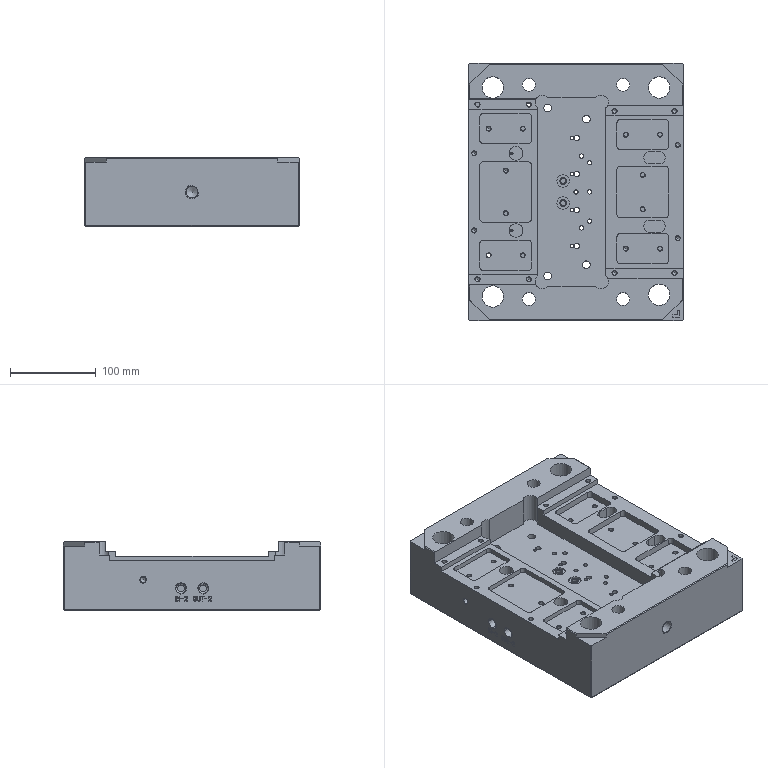NC program | PowerMill | posted with a generic post | part box 250 x 300 x 80 mm
Lines 1 to 768 of 17319:
%
O0001
N104 ( POWERMILL CB  : 2026004.0)
N105 ( POST VER      : 2026.0.0.5161)
N106 ( OPTION FILE   : FANUC)
N107 ( OUTPUT WORKPLANE : 1)
N108 (  )
N109 ( TOOL LIST )
N110 (----------------------------------)
N111 ( NO. | ID   | DIA.| TIP RAD|LENGTH)
N112 (----------------------------------)
N113 (    1|D8_1_1| 8.0 |  0.0   |100.24)
N114 (----------------------------------)
N115 (  )
N116 ( NUMBER OF TOOLPATHS: 1.0 )
N117 ( ESTIMATED PROGRAM DURATION: 0 HOURS 1 MIN 10 SEC)
N118 (  )
N119 G00 G21 G80 G40 G17
N120 G90
N121 G54
N122 G53 Z0.0
N123 (---------------)
N124 ( START TOOLPATH : 07中光-D8-等高 )
N125 (---------------)
N126 ( TOOL NO.    :1 )
N127 ( TOOL TYPE   : ENDMILL)
N128 ( TOOL ID     : D8_1_1)
N129 ( TOOL DIA    : 8.0 LENGTH 100.24)
N130 T1
N131 M6
N132 S3500 M03
N133 G00 G90 X82.0118 Y-12.1812
N134 G43 Z22.0 H1
N135
N136 G05 P10000 R8
N137 Z0.151
N138 G01 X82.0182 Y-12.2863 Z0.1455 F2100.0
N139 X82.0436 Y-12.4854 Z0.1349
N140 X82.0833 Y-12.687 Z0.1242
N141 X82.1478 Y-12.9174 Z0.1116
N142 X82.2928 Y-13.2849 Z0.0909
N143 X82.3993 Y-13.4891 Z0.0788
N144 X82.5476 Y-13.7209 Z0.0644
N145 X82.6911 Y-13.9087 Z0.052
N146 X82.9473 Y-14.183 Z0.0324
N147 X83.1294 Y-14.3414 Z0.0197
N148 X83.3239 Y-14.4841 Z0.0071
N149 X83.5429 Y-14.6176 Z-0.0064
N150 X83.7468 Y-14.721 Z-0.0183
N151 X83.9442 Y-14.8037 Z-0.0296
N152 X84.1906 Y-14.8839 Z-0.0431
N153 X84.5463 Y-14.9624 Z-0.0622
N154 X84.7454 Y-14.9854 Z-0.0727
N155 X84.946 Y-14.9952 Z-0.0833
N156 X85.1462 Y-14.9917 Z-0.0938
N157 X85.3458 Y-14.9751 Z-0.1042
N158 X85.5469 Y-14.9448 Z-0.1149
N159 X85.8094 Y-14.8839 Z-0.129
N160 X86.1453 Y-14.7681 F3500.0
N161 X86.3491 Y-14.6747
N162 X86.545 Y-14.5665
N163 X86.6761 Y-14.4841
N164 X86.9448 Y-14.2779
N165 X87.1514 Y-14.0844
N166 X87.3445 Y-13.8667
N167 X87.4785 Y-13.6846
N168 X87.6007 Y-13.4891
N169 X87.7443 Y-13.1999
N170 X87.8634 Y-12.8851
N171 X87.9167 Y-12.6871
N172 X87.9565 Y-12.4854
N173 X87.9818 Y-12.2863
N174 X87.994 Y-12.0857
N175 X87.9929 Y-11.8855
N176 X87.9787 Y-11.6859
N177 X87.9508 Y-11.4848
N178 X87.9095 Y-11.2862
N179 X87.8526 Y-11.0839
N180 X87.7443 Y-10.8001
N181 X87.5864 Y-10.4867
N182 X87.4717 Y-10.3056
N183 X87.3052 Y-10.0869
N184 X87.1326 Y-9.8969
N185 X86.9042 Y-9.6872
N186 X86.7294 Y-9.5539
N187 X86.545 Y-9.4335
N188 X86.2725 Y-9.2874
N189 X85.9478 Y-9.1585
N190 X85.7455 Y-9.099
N191 X85.5469 Y-9.0552
N192 X85.3458 Y-9.0249
N193 X85.1462 Y-9.0083
N194 X84.946 Y-9.0048
N195 X84.7454 Y-9.0146
N196 X84.5463 Y-9.0376
N197 X84.1466 Y-9.1279
N198 X83.9442 Y-9.1963
N199 X83.7274 Y-9.2874
N200 X83.5335 Y-9.3874
N201 X83.3471 Y-9.5013
N202 X83.0958 Y-9.6872
N203 X82.9473 Y-9.817
N204 X82.6949 Y-10.0869
N205 X82.5476 Y-10.2791
N206 X82.4136 Y-10.4867
N207 X82.3085 Y-10.6827
N208 X82.2181 Y-10.8864
N209 X82.1478 Y-11.0827
N210 X82.0905 Y-11.2862
N211 X82.0492 Y-11.4848
N212 X82.0213 Y-11.6859
N213 X82.0071 Y-11.8855
N214 X82.006 Y-12.0857
N215 X82.0182 Y-12.2863
N216 X82.0436 Y-12.4854
N217 X82.0833 Y-12.687
N218 X82.1478 Y-12.9174
N219 X82.2928 Y-13.2849
N220 X82.3993 Y-13.4891
N221 X82.5476 Y-13.7209
N222 X82.6911 Y-13.9087
N223 X82.9473 Y-14.183
N224 X83.1294 Y-14.3414
N225 X83.3239 Y-14.4841
N226 X83.5429 Y-14.6176
N227 X83.7468 Y-14.721
N228 X83.9442 Y-14.8037
N229 X84.1906 Y-14.8839
N230 X84.5463 Y-14.9624
N231 X84.7454 Y-14.9854
N232 X84.946 Y-14.9952
N233 X85.1462 Y-14.9917
N234 X85.3458 Y-14.9751
N235 X85.5469 Y-14.9448
N236 X85.8094 Y-14.8839
N237 X85.979 Y-14.8306 Z-0.1307
N238 X86.1485 Y-14.7667 Z-0.1324
N239 X86.3491 Y-14.6747 Z-0.1345
N240 X86.5471 Y-14.5652 Z-0.1366
N241 X86.6761 Y-14.4841 Z-0.1381
N242 X86.9481 Y-14.275 Z-0.1413
N243 X87.1513 Y-14.0844 Z-0.1439
N244 X87.3467 Y-13.8639 Z-0.1467
N245 X87.4785 Y-13.6846 Z-0.1488
N246 X87.6007 Y-13.4891 Z-0.151
N247 X87.7464 Y-13.1951 Z-0.1541
N248 X87.8634 Y-12.8851 Z-0.1572
N249 X87.9167 Y-12.6871 Z-0.1591
N250 X87.9564 Y-12.4854 Z-0.1611
N251 X87.9818 Y-12.2863 Z-0.163
N252 X87.994 Y-12.0857 Z-0.1649
N253 X87.9929 Y-11.8855 Z-0.1667
N254 X87.9787 Y-11.6859 Z-0.1686
N255 X87.9508 Y-11.4848 Z-0.1705
N256 X87.9095 Y-11.2862 Z-0.1725
N257 X87.8526 Y-11.0839 Z-0.1744
N258 X87.7819 Y-10.8864 Z-0.1764
N259 X87.6695 Y-10.6412 Z-0.179
N260 X87.5864 Y-10.4867 Z-0.1806
N261 X87.4717 Y-10.3056 Z-0.1826
N262 X87.3445 Y-10.1333 Z-0.1846
N263 X87.1326 Y-9.8969 Z-0.1876
N264 X86.9042 Y-9.6872 Z-0.1906
N265 X86.7294 Y-9.5539 Z-0.1926
N266 X86.545 Y-9.4335 Z-0.1947
N267 X86.2725 Y-9.2874 Z-0.1976
N268 X85.9478 Y-9.1585 Z-0.2009
N269 X85.7455 Y-9.099 Z-0.2029
N270 X85.5469 Y-9.0552 Z-0.2048
N271 X85.3458 Y-9.0249 Z-0.2067
N272 X85.1462 Y-9.0083 Z-0.2086
N273 X84.9429 Y-9.0049 Z-0.2106
N274 X84.7454 Y-9.0146 Z-0.2124
N275 X84.5463 Y-9.0376 Z-0.2143
N276 X84.3432 Y-9.076 Z-0.2163
N277 X84.1433 Y-9.1288 Z-0.2182
N278 X83.9442 Y-9.1963 Z-0.2202
N279 X83.7274 Y-9.2874 Z-0.2224
N280 X83.5305 Y-9.389 Z-0.2245
N281 X83.345 Y-9.5026 Z-0.2265
N282 X83.0958 Y-9.6872 Z-0.2295
N283 X82.9432 Y-9.8211 Z-0.2314
N284 X82.8145 Y-9.9498 Z-0.2331
N285 X82.6949 Y-10.0869 Z-0.2348
N286 X82.5453 Y-10.2822 Z-0.2371
N287 X82.4136 Y-10.4867 Z-0.2394
N288 X82.3085 Y-10.6827 Z-0.2415
N289 X82.2181 Y-10.8864 Z-0.2436
N290 X82.1467 Y-11.0858 Z-0.2456
N291 X82.0905 Y-11.2862 Z-0.2476
N292 X82.0492 Y-11.4848 Z-0.2495
N293 X82.0213 Y-11.6859 Z-0.2514
N294 X82.0071 Y-11.8855 Z-0.2533
N295 X82.006 Y-12.0857 Z-0.2552
N296 X82.0182 Y-12.2863 Z-0.2571
N297 X82.0436 Y-12.4854 Z-0.259
N298 X82.0833 Y-12.687 Z-0.2609
N299 X82.1366 Y-12.8851 Z-0.2628
N300 X82.2075 Y-13.0878 Z-0.2649
N301 X82.2928 Y-13.2849 Z-0.2669
N302 X82.3993 Y-13.4891 Z-0.2691
N303 X82.5215 Y-13.6846 Z-0.2712
N304 X82.6911 Y-13.9087 Z-0.2739
N305 X82.9473 Y-14.183 Z-0.2774
N306 X83.1294 Y-14.3414 Z-0.2797
N307 X83.3239 Y-14.4841 Z-0.282
N308 X83.546 Y-14.6192 Z-0.2844
N309 X83.7499 Y-14.7223 Z-0.2866
N310 X83.9442 Y-14.8037 Z-0.2886
N311 X84.1466 Y-14.8721 Z-0.2906
N312 X84.3449 Y-14.9243 Z-0.2925
N313 X84.5463 Y-14.9624 Z-0.2944
N314 X84.7454 Y-14.9854 Z-0.2963
N315 X84.946 Y-14.9952 Z-0.2982
N316 X85.1462 Y-14.9917 Z-0.3001
N317 X85.3458 Y-14.9751 Z-0.302
N318 X85.5469 Y-14.9448 Z-0.3039
N319 X85.8094 Y-14.8839 Z-0.3065
N320 X85.979 Y-14.8306 Z-0.3081
N321 X86.1485 Y-14.7667 Z-0.3098
N322 X86.3521 Y-14.6731 Z-0.3119
N323 X86.5471 Y-14.5652 Z-0.314
N324 X86.6761 Y-14.4841 Z-0.3155
N325 X86.9481 Y-14.275 Z-0.3187
N326 X87.1513 Y-14.0844 Z-0.3213
N327 X87.3467 Y-13.8639 Z-0.3241
N328 X87.4785 Y-13.6846 Z-0.3262
N329 X87.6007 Y-13.4891 Z-0.3284
N330 X87.7464 Y-13.1951 Z-0.3315
N331 X87.8634 Y-12.8851 Z-0.3346
N332 X87.9167 Y-12.6871 Z-0.3365
N333 X87.9564 Y-12.4854 Z-0.3385
N334 X87.9818 Y-12.2863 Z-0.3404
N335 X87.994 Y-12.0857 Z-0.3423
N336 X87.9929 Y-11.8855 Z-0.3442
N337 X87.9787 Y-11.6859 Z-0.346
N338 X87.9508 Y-11.4848 Z-0.348
N339 X87.9095 Y-11.2862 Z-0.3499
N340 X87.8526 Y-11.0839 Z-0.3519
N341 X87.7819 Y-10.8864 Z-0.3538
N342 X87.6695 Y-10.6412 Z-0.3564
N343 X87.5864 Y-10.4867 Z-0.358
N344 X87.4717 Y-10.3056 Z-0.36
N345 X87.3445 Y-10.1333 Z-0.3621
N346 X87.1326 Y-9.8969 Z-0.3651
N347 X86.9042 Y-9.6872 Z-0.368
N348 X86.7294 Y-9.5539 Z-0.3701
N349 X86.545 Y-9.4335 Z-0.3721
N350 X86.2725 Y-9.2874 Z-0.375
N351 X85.9478 Y-9.1585 Z-0.3783
N352 X85.7455 Y-9.099 Z-0.3803
N353 X85.5469 Y-9.0552 Z-0.3822
N354 X85.3458 Y-9.0249 Z-0.3842
N355 X85.1462 Y-9.0083 Z-0.3861
N356 X84.9429 Y-9.0049 Z-0.388
N357 X84.7454 Y-9.0146 Z-0.3898
N358 X84.54 Y-9.0388 Z-0.3918
N359 X84.3401 Y-9.0766 Z-0.3937
N360 X84.1433 Y-9.1288 Z-0.3956
N361 X83.9442 Y-9.1963 Z-0.3976
N362 X83.7274 Y-9.2874 Z-0.3998
N363 X83.5335 Y-9.3874 Z-0.4019
N364 X83.345 Y-9.5026 Z-0.404
N365 X83.0958 Y-9.6872 Z-0.4069
N366 X82.9432 Y-9.8211 Z-0.4088
N367 X82.8145 Y-9.9498 Z-0.4105
N368 X82.6949 Y-10.0869 Z-0.4122
N369 X82.5453 Y-10.2822 Z-0.4145
N370 X82.4136 Y-10.4867 Z-0.4168
N371 X82.3085 Y-10.6827 Z-0.4189
N372 X82.2181 Y-10.8864 Z-0.421
N373 X82.1478 Y-11.0827 Z-0.423
N374 X82.0905 Y-11.2862 Z-0.425
N375 X82.0492 Y-11.4848 Z-0.4269
N376 X82.0213 Y-11.6859 Z-0.4288
N377 X82.0071 Y-11.8855 Z-0.4307
N378 X82.006 Y-12.0857 Z-0.4326
N379 X82.0182 Y-12.2863 Z-0.4345
N380 X82.0436 Y-12.4854 Z-0.4364
N381 X82.0833 Y-12.687 Z-0.4383
N382 X82.1366 Y-12.8851 Z-0.4403
N383 X82.2075 Y-13.0878 Z-0.4423
N384 X82.2928 Y-13.2849 Z-0.4443
N385 X82.3993 Y-13.4891 Z-0.4465
N386 X82.5215 Y-13.6846 Z-0.4486
N387 X82.6911 Y-13.9087 Z-0.4513
N388 X82.9473 Y-14.183 Z-0.4548
N389 X83.1294 Y-14.3414 Z-0.4571
N390 X83.3239 Y-14.4841 Z-0.4594
N391 X83.5428 Y-14.6176 Z-0.4618
N392 X83.7468 Y-14.721 Z-0.464
N393 X83.9442 Y-14.8037 Z-0.466
N394 X84.1466 Y-14.8721 Z-0.468
N395 X84.3449 Y-14.9243 Z-0.4699
N396 X84.5463 Y-14.9624 Z-0.4719
N397 X84.7454 Y-14.9854 Z-0.4737
N398 X84.946 Y-14.9952 Z-0.4756
N399 X85.1462 Y-14.9917 Z-0.4775
N400 X85.3489 Y-14.9747 Z-0.4794
N401 X85.5469 Y-14.9448 Z-0.4813
N402 X85.8094 Y-14.8839 Z-0.4839
N403 X85.979 Y-14.8306 Z-0.4855
N404 X86.1485 Y-14.7667 Z-0.4873
N405 X86.3491 Y-14.6747 Z-0.4893
N406 X86.545 Y-14.5665 Z-0.4914
N407 X86.6761 Y-14.4841 Z-0.4929
N408 X86.9481 Y-14.275 Z-0.4961
N409 X87.1513 Y-14.0844 Z-0.4988
N410 X87.3445 Y-13.8667 Z-0.5015
N411 X87.4785 Y-13.6846 Z-0.5036
N412 X87.6007 Y-13.4891 Z-0.5058
N413 X87.7443 Y-13.1999 Z-0.5089
N414 X87.8634 Y-12.8851 Z-0.512
N415 X87.9167 Y-12.6871 Z-0.514
N416 X87.9564 Y-12.4854 Z-0.5159
N417 X87.9822 Y-12.2831 Z-0.5178
N418 X87.994 Y-12.0857 Z-0.5197
N419 X87.9929 Y-11.8855 Z-0.5216
N420 X87.9787 Y-11.6859 Z-0.5235
N421 X87.9508 Y-11.4848 Z-0.5254
N422 X87.9095 Y-11.2862 Z-0.5273
N423 X87.8526 Y-11.0839 Z-0.5293
N424 X87.7819 Y-10.8864 Z-0.5313
N425 X87.6695 Y-10.6412 Z-0.5338
N426 X87.5864 Y-10.4867 Z-0.5354
N427 X87.4717 Y-10.3056 Z-0.5375
N428 X87.3439 Y-10.1326 Z-0.5395
N429 X87.1326 Y-9.8969 Z-0.5425
N430 X86.9016 Y-9.685 Z-0.5454
N431 X86.7294 Y-9.5539 Z-0.5475
N432 X86.545 Y-9.4335 Z-0.5496
N433 X86.2705 Y-9.2866 Z-0.5525
N434 X85.9478 Y-9.1585 Z-0.5558
N435 X85.7455 Y-9.099 Z-0.5578
N436 X85.5469 Y-9.0552 Z-0.5597
N437 X85.3458 Y-9.0249 Z-0.5616
N438 X85.1462 Y-9.0083 Z-0.5635
N439 X84.9429 Y-9.0049 Z-0.5654
N440 X84.7454 Y-9.0146 Z-0.5673
N441 X84.54 Y-9.0388 Z-0.5692
N442 X84.3417 Y-9.0763 Z-0.5711
N443 X84.1466 Y-9.1279 Z-0.573
N444 X83.9442 Y-9.1963 Z-0.575
N445 X83.7274 Y-9.2875 Z-0.5772
N446 X83.5305 Y-9.389 Z-0.5793
N447 X83.345 Y-9.5026 Z-0.5814
N448 X83.0958 Y-9.6872 Z-0.5843
N449 X82.9432 Y-9.8211 Z-0.5862
N450 X82.8145 Y-9.9498 Z-0.5879
N451 X82.6949 Y-10.0869 Z-0.5896
N452 X82.5476 Y-10.2791 Z-0.5919
N453 X82.4136 Y-10.4867 Z-0.5943
N454 X82.3085 Y-10.6827 Z-0.5964
N455 X82.2181 Y-10.8864 Z-0.5985
N456 X82.1478 Y-11.0827 Z-0.6004
N457 X82.0905 Y-11.2862 Z-0.6024
N458 X82.0492 Y-11.4848 Z-0.6043
N459 X82.0213 Y-11.6859 Z-0.6062
N460 X82.0071 Y-11.8855 Z-0.6081
N461 X82.006 Y-12.0857 Z-0.61
N462 X82.0182 Y-12.2863 Z-0.6119
N463 X82.0436 Y-12.4854 Z-0.6138
N464 X82.0833 Y-12.687 Z-0.6157
N465 X82.1366 Y-12.8851 Z-0.6177
N466 X82.2075 Y-13.0878 Z-0.6197
N467 X82.2928 Y-13.2849 Z-0.6217
N468 X82.3993 Y-13.4891 Z-0.6239
N469 X82.5215 Y-13.6846 Z-0.6261
N470 X82.6911 Y-13.9087 Z-0.6287
N471 X82.9473 Y-14.183 Z-0.6323
N472 X83.1294 Y-14.3414 Z-0.6345
N473 X83.3239 Y-14.4841 Z-0.6368
N474 X83.5428 Y-14.6176 Z-0.6392
N475 X83.7468 Y-14.721 Z-0.6414
N476 X83.9473 Y-14.8048 Z-0.6434
N477 X84.1473 Y-14.8723 Z-0.6454
N478 X84.3452 Y-14.9244 Z-0.6473
N479 X84.5463 Y-14.9624 Z-0.6493
N480 X84.7454 Y-14.9854 Z-0.6512
N481 X84.946 Y-14.9952 Z-0.6531
N482 X85.1462 Y-14.9917 Z-0.6549
N483 X85.3489 Y-14.9747 Z-0.6569
N484 X85.5469 Y-14.9448 Z-0.6587
N485 X85.8094 Y-14.8839 Z-0.6613
N486 X86.1453 Y-14.7681 Z-0.6646
N487 X86.3491 Y-14.6747 Z-0.6668
N488 X86.545 Y-14.5665 Z-0.6689
N489 X86.6761 Y-14.4841 Z-0.6703
N490 X86.9448 Y-14.2779 Z-0.6735
N491 X87.1513 Y-14.0844 Z-0.6762
N492 X87.3445 Y-13.8667 Z-0.6789
N493 X87.4785 Y-13.6846 Z-0.6811
N494 X87.6024 Y-13.4859 Z-0.6833
N495 X87.7464 Y-13.1951 Z-0.6863
N496 X87.8634 Y-12.8851 Z-0.6895
N497 X87.9175 Y-12.684 Z-0.6914
N498 X87.9564 Y-12.4854 Z-0.6933
N499 X87.9822 Y-12.2831 Z-0.6952
N500 X87.994 Y-12.0857 Z-0.6971
N501 X87.9929 Y-11.8855 Z-0.699
N502 X87.9787 Y-11.6859 Z-0.7009
N503 X87.9508 Y-11.4848 Z-0.7028
N504 X87.9086 Y-11.283 Z-0.7047
N505 X87.8515 Y-11.0808 Z-0.7067
N506 X87.7813 Y-10.8851 Z-0.7087
N507 X87.6683 Y-10.6388 Z-0.7112
N508 X87.5846 Y-10.4838 Z-0.7129
N509 X87.4717 Y-10.3056 Z-0.7149
N510 X87.3445 Y-10.1333 Z-0.7169
N511 X87.1298 Y-9.8941 Z-0.7199
N512 X86.9042 Y-9.6872 Z-0.7228
N513 X86.7294 Y-9.5539 Z-0.7249
N514 X86.543 Y-9.4322 Z-0.727
N515 X86.2725 Y-9.2874 Z-0.7299
N516 X85.9478 Y-9.1585 Z-0.7332
N517 X85.7425 Y-9.0982 Z-0.7352
N518 X85.5469 Y-9.0552 Z-0.7371
N519 X85.3427 Y-9.0246 Z-0.739
N520 X85.1462 Y-9.0083 Z-0.7409
N521 X84.946 Y-9.0048 Z-0.7428
N522 X84.7454 Y-9.0146 Z-0.7447
N523 X84.5463 Y-9.0376 Z-0.7466
N524 X84.3448 Y-9.0757 Z-0.7485
N525 X84.1466 Y-9.1279 Z-0.7504
N526 X83.9442 Y-9.1963 Z-0.7524
N527 X83.7275 Y-9.2874 Z-0.7547
N528 X83.5335 Y-9.3874 Z-0.7567
N529 X83.3471 Y-9.5013 Z-0.7588
N530 X83.0958 Y-9.6872 Z-0.7617
N531 X82.9473 Y-9.817 Z-0.7636
N532 X82.8165 Y-9.9478 Z-0.7653
N533 X82.6949 Y-10.0869 Z-0.7671
N534 X82.5476 Y-10.2791 Z-0.7693
N535 X82.4136 Y-10.4867 Z-0.7717
N536 X82.3085 Y-10.6827 Z-0.7738
N537 X82.2181 Y-10.8864 Z-0.7759
N538 X82.1478 Y-11.0827 Z-0.7778
N539 X82.0905 Y-11.2862 Z-0.7798
N540 X82.0487 Y-11.4879 Z-0.7818
N541 X82.0213 Y-11.6859 Z-0.7837
N542 X82.007 Y-11.8887 Z-0.7856
N543 X82.0061 Y-12.0888 Z-0.7875
N544 X82.0182 Y-12.2863 Z-0.7893
N545 X82.0436 Y-12.4854 Z-0.7912
N546 X82.0833 Y-12.687 Z-0.7932
N547 X82.1367 Y-12.8857 Z-0.7951
N548 X82.2076 Y-13.0881 Z-0.7971
N549 X82.2928 Y-13.2849 Z-0.7991
N550 X82.3993 Y-13.4891 Z-0.8013
N551 X82.5219 Y-13.6852 Z-0.8035
N552 X82.6911 Y-13.9087 Z-0.8061
N553 X82.95 Y-14.1857 Z-0.8097
N554 X83.1323 Y-14.3437 Z-0.812
N555 X83.3239 Y-14.4841 Z-0.8142
N556 X83.5428 Y-14.6176 Z-0.8166
N557 X83.7499 Y-14.7223 Z-0.8188
N558 X83.9442 Y-14.8037 Z-0.8208
N559 X84.1796 Y-14.8809 Z-0.8232
N560 X84.3632 Y-14.9278 Z-0.8249
N561 X84.5494 Y-14.963 Z-0.8267
N562 X84.7454 Y-14.9854 Z-0.8286
N563 X84.946 Y-14.9952 Z-0.8305
N564 X85.1462 Y-14.9917 Z-0.8324
N565 X85.3458 Y-14.9751 Z-0.8343
N566 X85.5469 Y-14.9448 Z-0.8362
N567 X85.8094 Y-14.8839 Z-0.8387
N568 X86.1453 Y-14.7681 Z-0.8421
N569 X86.3491 Y-14.6747 Z-0.8442
N570 X86.545 Y-14.5665 Z-0.8463
N571 X86.6761 Y-14.4841 Z-0.8477
N572 X86.9448 Y-14.2779 Z-0.8509
N573 X87.1513 Y-14.0844 Z-0.8536
N574 X87.3445 Y-13.8667 Z-0.8563
N575 X87.4785 Y-13.6846 Z-0.8585
N576 X87.6007 Y-13.4891 Z-0.8607
N577 X87.7443 Y-13.1999 Z-0.8637
N578 X87.8634 Y-12.8851 Z-0.8669
N579 X87.9167 Y-12.6871 Z-0.8688
N580 X87.9564 Y-12.4854 Z-0.8707
N581 X87.9818 Y-12.2863 Z-0.8726
N582 X87.994 Y-12.0857 Z-0.8745
N583 X87.9929 Y-11.8855 Z-0.8764
N584 X87.9783 Y-11.6828 Z-0.8783
N585 X87.9502 Y-11.4817 Z-0.8802
N586 X87.9095 Y-11.2862 Z-0.8821
N587 X87.8526 Y-11.0839 Z-0.8841
N588 X87.7819 Y-10.8864 Z-0.8861
N589 X87.6683 Y-10.6388 Z-0.8887
N590 X87.5864 Y-10.4867 Z-0.8903
N591 X87.4717 Y-10.3056 Z-0.8923
N592 X87.3439 Y-10.1326 Z-0.8943
N593 X87.1326 Y-9.8969 Z-0.8973
N594 X86.9042 Y-9.6872 Z-0.9002
N595 X86.7294 Y-9.5539 Z-0.9023
N596 X86.543 Y-9.4322 Z-0.9044
N597 X86.2725 Y-9.2874 Z-0.9073
N598 X85.9478 Y-9.1585 Z-0.9106
N599 X85.7425 Y-9.0982 Z-0.9126
N600 X85.5469 Y-9.0552 Z-0.9145
N601 X85.3427 Y-9.0246 Z-0.9165
N602 X85.1462 Y-9.0083 Z-0.9183
N603 X84.946 Y-9.0048 Z-0.9202
N604 X84.7454 Y-9.0146 Z-0.9221
N605 X84.54 Y-9.0388 Z-0.924
N606 X84.3401 Y-9.0766 Z-0.926
N607 X84.1433 Y-9.1288 Z-0.9279
N608 X83.9442 Y-9.1963 Z-0.9299
N609 X83.7275 Y-9.2874 Z-0.9321
N610 X83.5335 Y-9.3874 Z-0.9341
N611 X83.3471 Y-9.5013 Z-0.9362
N612 X83.0958 Y-9.6872 Z-0.9391
N613 X82.9473 Y-9.817 Z-0.941
N614 X82.8165 Y-9.9478 Z-0.9427
N615 X82.6949 Y-10.0869 Z-0.9445
N616 X82.5476 Y-10.2791 Z-0.9468
N617 X82.4136 Y-10.4867 Z-0.9491
N618 X82.3085 Y-10.6827 Z-0.9512
N619 X82.2181 Y-10.8864 Z-0.9533
N620 X82.1478 Y-11.0827 Z-0.9553
N621 X82.0905 Y-11.2862 Z-0.9573
N622 X82.0492 Y-11.4848 Z-0.9592
N623 X82.0213 Y-11.6859 Z-0.9611
N624 X82.0071 Y-11.8855 Z-0.963
N625 X82.006 Y-12.0857 Z-0.9649
N626 X82.0182 Y-12.2863 Z-0.9667
N627 X82.0442 Y-12.4886 Z-0.9687
N628 X82.0833 Y-12.687 Z-0.9706
N629 X82.1366 Y-12.8851 Z-0.9725
N630 X82.2081 Y-13.0895 Z-0.9746
N631 X82.2943 Y-13.2882 Z-0.9766
N632 X82.3993 Y-13.4891 Z-0.9787
N633 X82.5215 Y-13.6846 Z-0.9809
N634 X82.6911 Y-13.9087 Z-0.9836
N635 X82.9473 Y-14.183 Z-0.9871
N636 X83.1294 Y-14.3414 Z-0.9894
N637 X83.3239 Y-14.4841 Z-0.9916
N638 X83.546 Y-14.6192 Z-0.9941
N639 X83.7468 Y-14.721 Z-0.9962
N640 X83.9442 Y-14.8037 Z-0.9982
N641 X84.1472 Y-14.8723 Z-1.0003
N642 X84.3467 Y-14.9246 Z-1.0022
N643 X84.5494 Y-14.963 Z-1.0041
N644 X84.7454 Y-14.9854 Z-1.006
N645 X84.946 Y-14.9952 Z-1.0079
N646 X85.1462 Y-14.9917 Z-1.0098
N647 X85.3458 Y-14.9751 Z-1.0117
N648 X85.5469 Y-14.9448 Z-1.0136
N649 X85.8094 Y-14.8839 Z-1.0161
N650 X86.1453 Y-14.7681 Z-1.0195
N651 X86.3491 Y-14.6747 Z-1.0216
N652 X86.545 Y-14.5665 Z-1.0237
N653 X86.6761 Y-14.4841 Z-1.0252
N654 X86.9448 Y-14.2779 Z-1.0284
N655 X87.1513 Y-14.0844 Z-1.031
N656 X87.3445 Y-13.8667 Z-1.0338
N657 X87.4785 Y-13.6846 Z-1.0359
N658 X87.6007 Y-13.4891 Z-1.0381
N659 X87.7443 Y-13.1999 Z-1.0411
N660 X87.8634 Y-12.8851 Z-1.0443
N661 X87.9167 Y-12.6871 Z-1.0462
N662 X87.9564 Y-12.4854 Z-1.0482
N663 X87.9818 Y-12.2863 Z-1.0501
N664 X87.994 Y-12.0857 Z-1.052
N665 X87.9929 Y-11.8855 Z-1.0538
N666 X87.9787 Y-11.6859 Z-1.0557
N667 X87.9508 Y-11.4848 Z-1.0576
N668 X87.9095 Y-11.2862 Z-1.0596
N669 X87.8526 Y-11.0839 Z-1.0615
N670 X87.7819 Y-10.8864 Z-1.0635
N671 X87.6695 Y-10.6412 Z-1.0661
N672 X87.5864 Y-10.4867 Z-1.0677
N673 X87.4717 Y-10.3056 Z-1.0697
N674 X87.3439 Y-10.1326 Z-1.0718
N675 X87.1326 Y-9.8969 Z-1.0747
N676 X86.9042 Y-9.6872 Z-1.0777
N677 X86.7294 Y-9.5539 Z-1.0797
N678 X86.545 Y-9.4335 Z-1.0818
N679 X86.2725 Y-9.2874 Z-1.0847
N680 X85.9478 Y-9.1585 Z-1.088
N681 X85.7455 Y-9.099 Z-1.09
N682 X85.5469 Y-9.0552 Z-1.0919
N683 X85.3458 Y-9.0249 Z-1.0938
N684 X85.1462 Y-9.0083 Z-1.0957
N685 X84.946 Y-9.0048 Z-1.0976
N686 X84.7454 Y-9.0146 Z-1.0995
N687 X84.54 Y-9.0388 Z-1.1015
N688 X84.3401 Y-9.0766 Z-1.1034
N689 X84.1433 Y-9.1288 Z-1.1053
N690 X83.9442 Y-9.1963 Z-1.1073
N691 X83.7275 Y-9.2874 Z-1.1095
N692 X83.5335 Y-9.3874 Z-1.1116
N693 X83.3471 Y-9.5013 Z-1.1136
N694 X83.0958 Y-9.6872 Z-1.1166
N695 X82.9432 Y-9.8211 Z-1.1185
N696 X82.8145 Y-9.9498 Z-1.1202
N697 X82.6949 Y-10.0869 Z-1.1219
N698 X82.5453 Y-10.2822 Z-1.1242
N699 X82.4136 Y-10.4867 Z-1.1265
N700 X82.3085 Y-10.6827 Z-1.1286
N701 X82.2181 Y-10.8864 Z-1.1307
N702 X82.1478 Y-11.0827 Z-1.1327
N703 X82.0905 Y-11.2862 Z-1.1347
N704 X82.0492 Y-11.4848 Z-1.1366
N705 X82.0213 Y-11.6859 Z-1.1385
N706 X82.0071 Y-11.8855 Z-1.1404
N707 X82.006 Y-12.0857 Z-1.1423
N708 X82.0182 Y-12.2863 Z-1.1442
N709 X82.0436 Y-12.4854 Z-1.1461
N710 X82.0833 Y-12.687 Z-1.148
N711 X82.1366 Y-12.8851 Z-1.1499
N712 X82.2075 Y-13.0878 Z-1.152
N713 X82.2928 Y-13.2849 Z-1.154
N714 X82.3993 Y-13.4891 Z-1.1561
N715 X82.5215 Y-13.6846 Z-1.1583
N716 X82.6935 Y-13.9115 Z-1.161
N717 X82.9473 Y-14.183 Z-1.1645
N718 X83.1294 Y-14.3414 Z-1.1668
N719 X83.3239 Y-14.4841 Z-1.1691
N720 X83.5428 Y-14.6176 Z-1.1715
N721 X83.7468 Y-14.721 Z-1.1736
N722 X83.9442 Y-14.8037 Z-1.1757
N723 X84.1466 Y-14.8721 Z-1.1777
N724 X84.3449 Y-14.9243 Z-1.1796
N725 X84.5463 Y-14.9624 Z-1.1815
N726 X84.7454 Y-14.9854 Z-1.1834
N727 X84.946 Y-14.9952 Z-1.1853
N728 X85.1462 Y-14.9917 Z-1.1872
N729 X85.3458 Y-14.9751 Z-1.1891
N730 X85.5469 Y-14.9448 Z-1.191
N731 X85.8094 Y-14.8839 Z-1.1935
N732 X85.979 Y-14.8306 Z-1.1952
N733 X86.1485 Y-14.7667 Z-1.1969
N734 X86.3521 Y-14.6731 Z-1.199
N735 X86.5471 Y-14.5652 Z-1.2011
N736 X86.6761 Y-14.4841 Z-1.2026
N737 X86.9481 Y-14.275 Z-1.2058
N738 X87.1513 Y-14.0844 Z-1.2084
N739 X87.3467 Y-13.8639 Z-1.2112
N740 X87.4785 Y-13.6846 Z-1.2133
N741 X87.6007 Y-13.4891 Z-1.2155
N742 X87.7464 Y-13.1951 Z-1.2186
N743 X87.8634 Y-12.8851 Z-1.2217
N744 X87.9167 Y-12.6871 Z-1.2236
N745 X87.9564 Y-12.4854 Z-1.2256
N746 X87.9818 Y-12.2863 Z-1.2275
N747 X87.994 Y-12.0857 Z-1.2294
N748 X87.9929 Y-11.8855 Z-1.2313
N749 X87.9787 Y-11.6859 Z-1.2331
N750 X87.9508 Y-11.4848 Z-1.2351
N751 X87.9095 Y-11.2862 Z-1.237
N752 X87.8526 Y-11.0839 Z-1.239
N753 X87.7819 Y-10.8864 Z-1.2409
N754 X87.6695 Y-10.6412 Z-1.2435
N755 X87.5864 Y-10.4867 Z-1.2451
N756 X87.4717 Y-10.3056 Z-1.2471
N757 X87.3445 Y-10.1333 Z-1.2492
N758 X87.1326 Y-9.8969 Z-1.2522
N759 X86.9042 Y-9.6872 Z-1.2551
N760 X86.7294 Y-9.5539 Z-1.2572
N761 X86.545 Y-9.4335 Z-1.2592
N762 X86.2725 Y-9.2874 Z-1.2621
N763 X85.9478 Y-9.1585 Z-1.2654
N764 X85.7455 Y-9.099 Z-1.2674
N765 X85.5469 Y-9.0552 Z-1.2693
N766 X85.3458 Y-9.0249 Z-1.2713
N767 X85.1462 Y-9.0083 Z-1.2732
N768 X84.9429 Y-9.0049 Z-1.2751
N769 X84.7454 Y-9.0146 Z-1.2769
N770 X84.54 Y-9.0388 Z-1.2789
N771 X84.3417 Y-9.0763 Z-1.2808
N772 X84.1466 Y-9.1279 Z-1.2827
N773 X83.9442 Y-9.1963 Z-1.2847
N774 X83.7275 Y-9.2874 Z-1.2869
N775 X83.5335 Y-9.3874 Z-1.289
N776 X83.345 Y-9.5026 Z-1.2911
N777 X83.0958 Y-9.6872 Z-1.294
N778 X82.9432 Y-9.8211 Z-1.2959
N779 X82.8145 Y-9.9498 Z-1.2976
N780 X82.6949 Y-10.0869 Z-1.2993
N781 X82.5453 Y-10.2822 Z-1.3016
N782 X82.4136 Y-10.4867 Z-1.3039
N783 X82.3085 Y-10.6827 Z-1.306
N784 X82.2181 Y-10.8864 Z-1.3081
N785 X82.1478 Y-11.0827 Z-1.3101
N786 X82.0905 Y-11.2862 Z-1.3121
N787 X82.0492 Y-11.4848 Z-1.314
N788 X82.0213 Y-11.6859 Z-1.3159
N789 X82.0071 Y-11.8855 Z-1.3178
N790 X82.006 Y-12.0857 Z-1.3197
N791 X82.0182 Y-12.2863 Z-1.3216
N792 X82.0436 Y-12.4854 Z-1.3235
N793 X82.0833 Y-12.687 Z-1.3254
N794 X82.1366 Y-12.8851 Z-1.3274
N795 X82.2075 Y-13.0878 Z-1.3294
N796 X82.2928 Y-13.2849 Z-1.3314
N797 X82.3993 Y-13.4891 Z-1.3336
N798 X82.5215 Y-13.6846 Z-1.3357
N799 X82.6911 Y-13.9087 Z-1.3384
N800 X82.9473 Y-14.183 Z-1.3419
N801 X83.1294 Y-14.3414 Z-1.3442
N802 X83.3239 Y-14.4841 Z-1.3465
N803 X83.5428 Y-14.6176 Z-1.3489
N804 X83.7468 Y-14.721 Z-1.3511
N805 X83.9442 Y-14.8037 Z-1.3531
N806 X84.1466 Y-14.8721 Z-1.3551
N807 X84.3449 Y-14.9243 Z-1.357
N808 X84.5463 Y-14.9624 Z-1.359
N809 X84.7454 Y-14.9854 Z-1.3608
N810 X84.946 Y-14.9952 Z-1.3627
N811 X85.1462 Y-14.9917 Z-1.3646
N812 X85.3489 Y-14.9747 Z-1.3665
N813 X85.5469 Y-14.9448 Z-1.3684
N814 X85.8094 Y-14.8839 Z-1.371
N815 X85.979 Y-14.8306 Z-1.3726
N816 X86.1485 Y-14.7667 Z-1.3744
N817 X86.3491 Y-14.6747 Z-1.3764
N818 X86.5471 Y-14.5652 Z-1.3786
N819 X86.6761 Y-14.4841 Z-1.38
N820 X86.9481 Y-14.275 Z-1.3832
N821 X87.1513 Y-14.0844 Z-1.3859
N822 X87.3467 Y-13.8639 Z-1.3886
N823 X87.4785 Y-13.6846 Z-1.3907
N824 X87.6007 Y-13.4891 Z-1.3929
N825 X87.7464 Y-13.1951 Z-1.396
N826 X87.8634 Y-12.8851 Z-1.3991
N827 X87.9167 Y-12.6871 Z-1.4011
N828 X87.9564 Y-12.4854 Z-1.403
N829 X87.9818 Y-12.2863 Z-1.4049
N830 X87.994 Y-12.0857 Z-1.4068
N831 X87.9929 Y-11.8855 Z-1.4087
N832 X87.9787 Y-11.6859 Z-1.4106
N833 X87.9508 Y-11.4848 Z-1.4125
N834 X87.9095 Y-11.2862 Z-1.4144
N835 X87.8526 Y-11.0839 Z-1.4164
N836 X87.7819 Y-10.8864 Z-1.4183
N837 X87.6695 Y-10.6412 Z-1.4209
N838 X87.5864 Y-10.4867 Z-1.4225
N839 X87.4717 Y-10.3056 Z-1.4246
N840 X87.3445 Y-10.1333 Z-1.4266
N841 X87.1326 Y-9.8969 Z-1.4296
N842 X86.9042 Y-9.6872 Z-1.4325
N843 X86.7266 Y-9.5518 Z-1.4346
N844 X86.543 Y-9.4322 Z-1.4367
N845 X86.2725 Y-9.2874 Z-1.4396
N846 X85.9478 Y-9.1585 Z-1.4429
N847 X85.7455 Y-9.099 Z-1.4448
N848 X85.5469 Y-9.0552 Z-1.4468
N849 X85.3458 Y-9.0249 Z-1.4487
N850 X85.1462 Y-9.0083 Z-1.4506
N851 X84.9429 Y-9.0049 Z-1.4525
N852 X84.7454 Y-9.0146 Z-1.4544
N853 X84.54 Y-9.0388 Z-1.4563
N854 X84.3401 Y-9.0766 Z-1.4582
N855 X84.1433 Y-9.1288 Z-1.4601
N856 X83.9442 Y-9.1963 Z-1.4621
N857 X83.7275 Y-9.2874 Z-1.4643
N858 X83.5335 Y-9.3874 Z-1.4664
N859 X83.345 Y-9.5026 Z-1.4685
N860 X83.0958 Y-9.6872 Z-1.4714
N861 X82.9432 Y-9.8211 Z-1.4733
N862 X82.8145 Y-9.9498 Z-1.475
N863 X82.6949 Y-10.0869 Z-1.4767
N864 X82.5453 Y-10.2822 Z-1.4791
N865 X82.4136 Y-10.4867 Z-1.4814